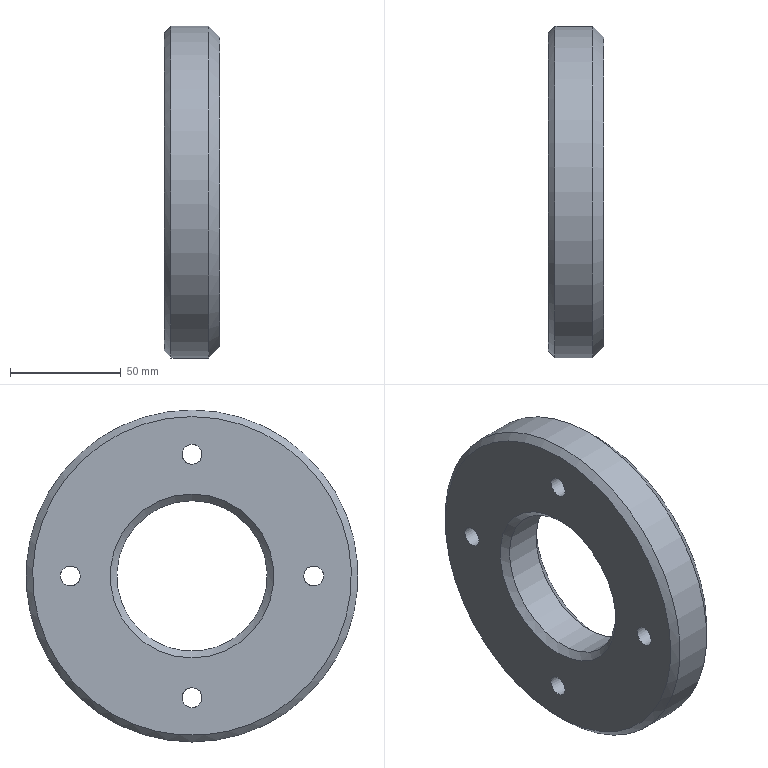Part | STEP file | solid 91 | 1 solid | 20 faces | box 25 x 150 x 150 mm | volume 329738 mm3 | cylinder 10 | plane 6 | cone 4 | commonest cylinder face diameters 9 x4 14 x4 68 x1 150 x1